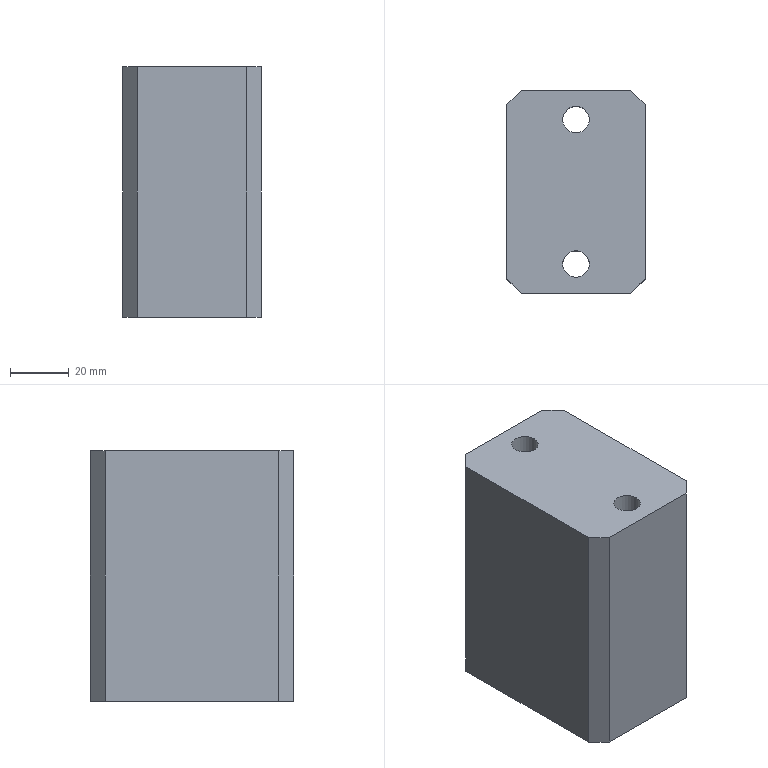Part | STEP file | 216_id1578_x_t | 1 solid | 22 faces | box 47 x 69 x 85 mm | volume 251605 mm3 | plane 12 | cylinder 6 | cone 4 | commonest cylinder face diameters 6.8 x2 9 x2 14 x2